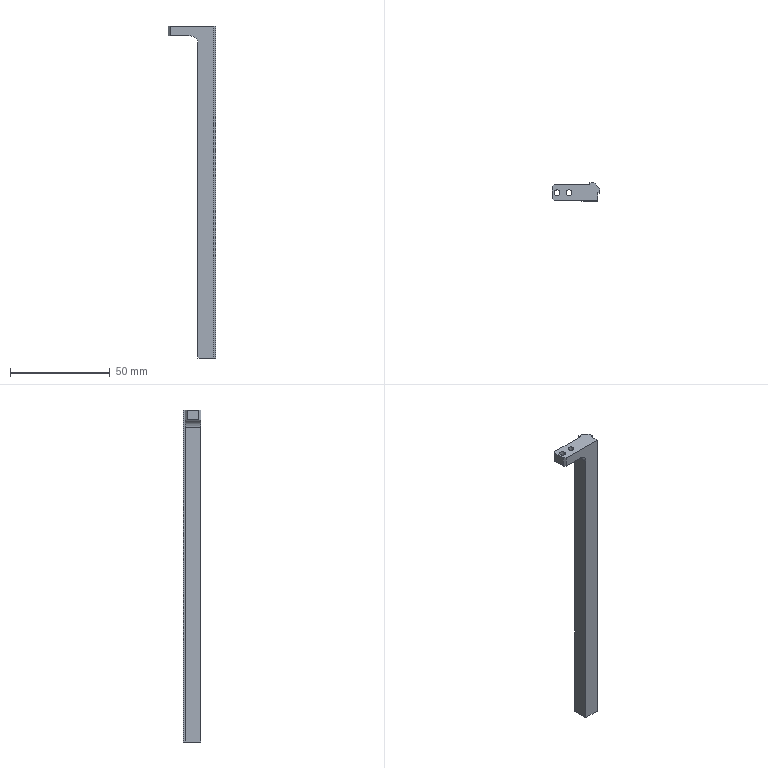Part | 1 solid | 62 faces | box 24 x 9 x 166.5 mm | volume 11877 mm3 | cone 28 | cylinder 19 | plane 15 | commonest cylinder face diameters 1.6 x14 2.9 x4 8 x1